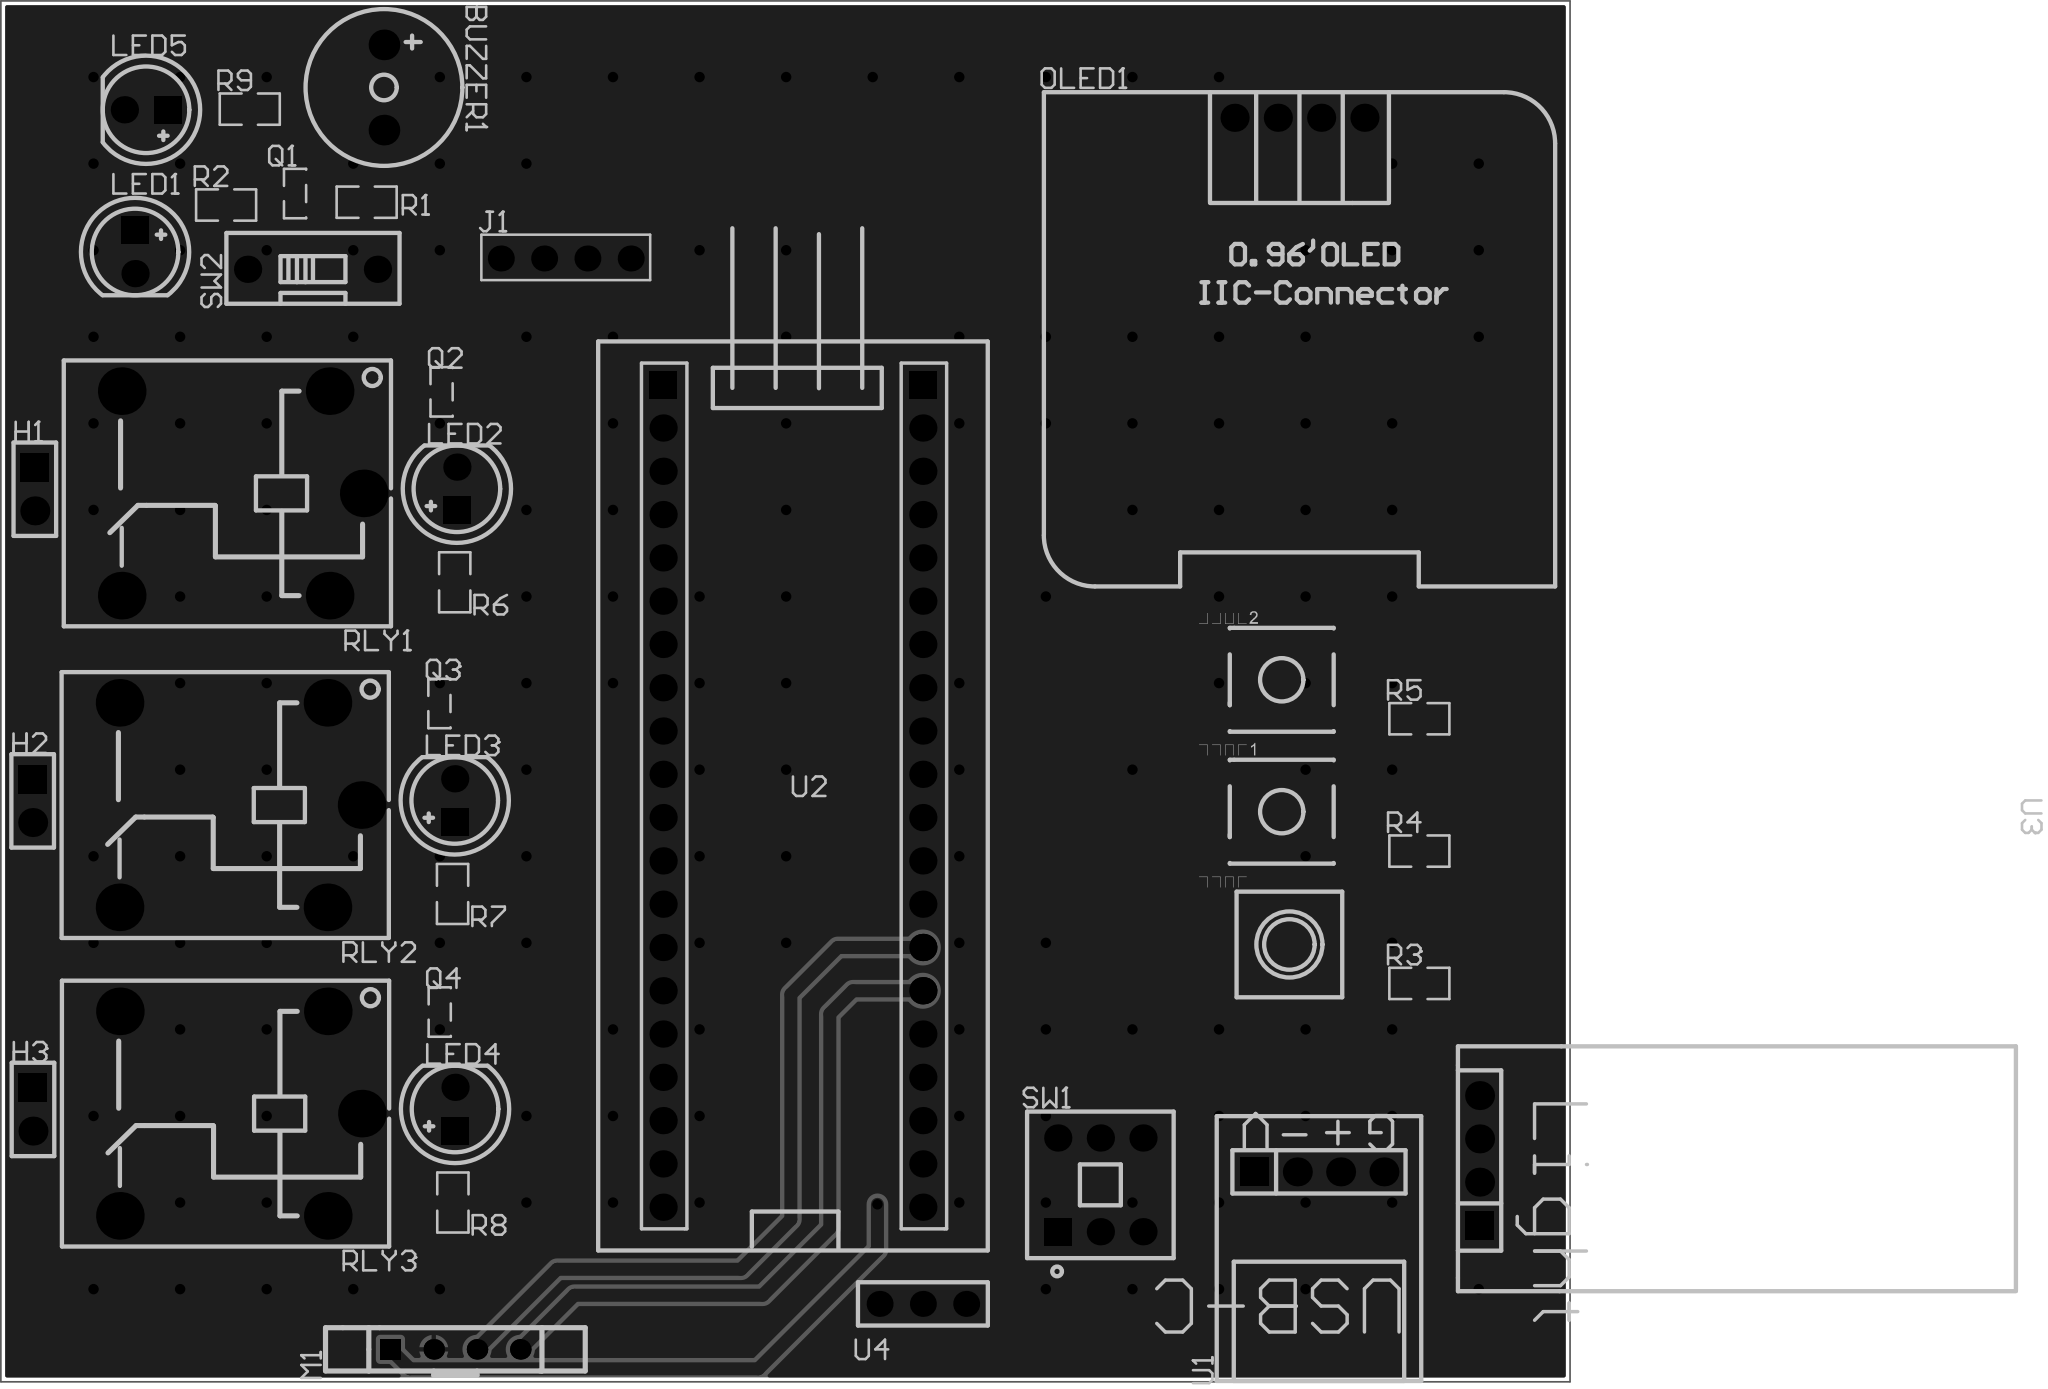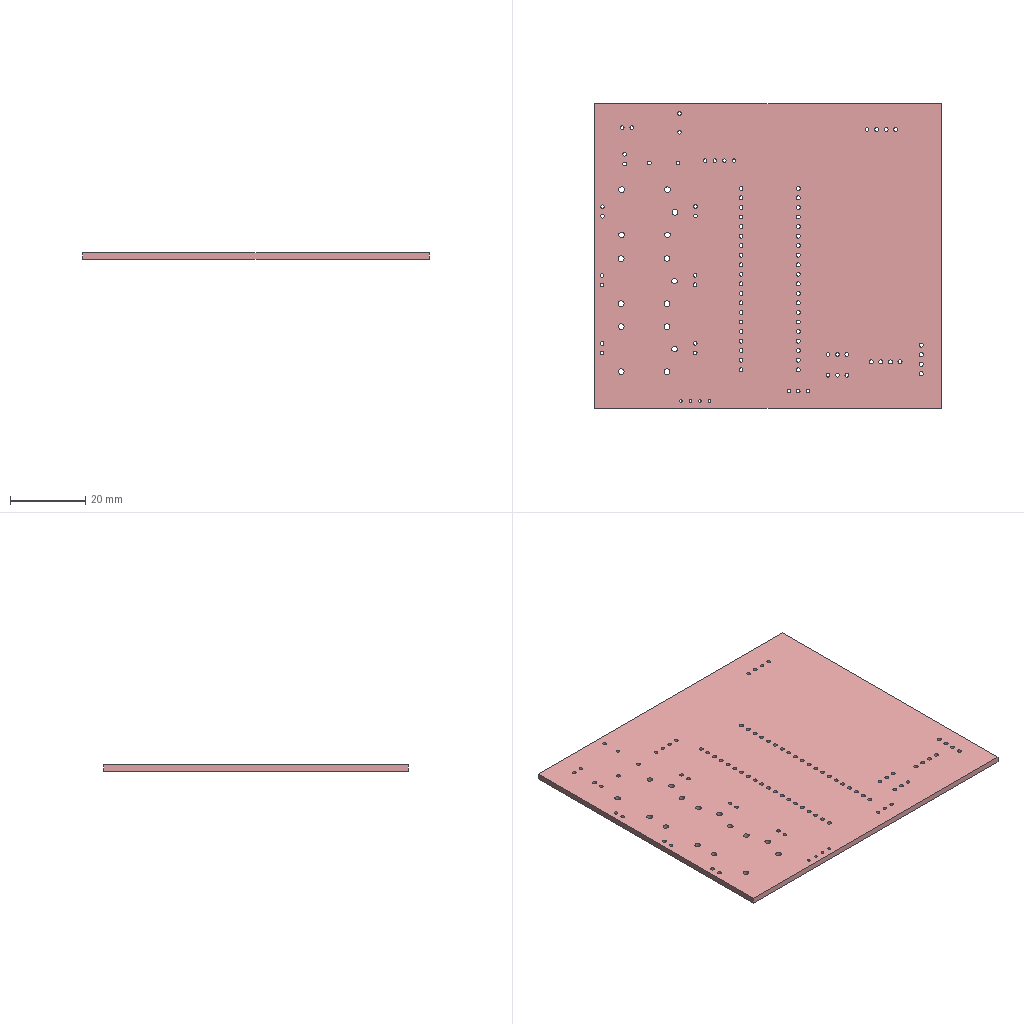Circuit board layout | Altium Designer | box 92.1 x 81 x 1.6 mm
Layer stack:
# Altium Designer layer stack of  (unit mm; dielectric type: 0 none, 1 core, 2 prepreg, 3 surface material)
index,name,kind,layer,copper_thickness_mm,dielectric_type,dielectric_thickness_mm,dielectric_material,dielectric_constant
0,Top Paste Mask Layer,other,,,,,,
1,Top Silkscreen Layer,other,,,,,,
2,Top Solder Mask Layer,dielectric,,,3,0.01,,3.3
3,Top Layer,copper,Top Layer,0.035,,,,
4,Dielectric1,dielectric,,,3,1.51,FR4,4.5
5,Bottom Layer,copper,Bottom Layer,0.035,,,,
6,Bottom Solder Mask Layer,dielectric,,,3,0.01,,3.3
7,Bottom Silkscreen Layer,other,,,,,,
8,Bottom Paste Mask Layer,other,,,,,,
# drill layer pairs: low layer,high layer
drill_pair,Top Layer,Bottom Layer
Part placement:
Designator,Comment,Layer,Footprint,Center-X(mm),Center-Y(mm),Rotation
BUZZER1,3kHz,TopLayer,BUZ-TH_BD9.0-P5.00-D0.6-FD,102.997,157.988,270
H1,,TopLayer,HDR-TH_2P-P2.54-V-F,82.511,134.416,270
H2,,TopLayer,HDR-TH_2P-P2.54-V-F,82.385,116.128,270
H3,,TopLayer,HDR-TH_2P-P2.54-V-F,82.403,98.024,270
J1,土壤湿度传感器模块,TopLayer,Hearder-4,113.665,147.955,0
LED1,,TopLayer,LED-TH_5mm,88.392,148.336,270
LED2,,TopLayer,LED-TH_5mm,107.276,134.443,90
LED3,,TopLayer,LED-TH_5mm,107.15,116.155,90
LED4,,TopLayer,LED-TH_5mm,107.168,98.051,90
LED5,,TopLayer,LED-TH_5mm,89.036,156.68,180
M1,BT06,TopLayer,BT06,107.188,83.947,90
OLED1,,TopLayer,0.96OLED_4P,156.718,156.21,0
Q1,S8050,TopLayer,SOT-23-3_L2.9-W1.3-P1.90-LS2.3-BR,97.79,151.765,0
Q2,S8050,TopLayer,SOT-23-3_L2.9-W1.3-P1.90-LS2.3-BR,106.388,140.131,0
Q3,S8050,TopLayer,SOT-23-3_L2.9-W1.3-P1.90-LS2.3-BR,106.26,121.843,0
Q4,S8050,TopLayer,SOT-23-3_L2.9-W1.3-P1.90-LS2.3-BR,106.279,103.739,0
R1,1K,TopLayer,R0805,101.981,151.257,180
R2,1K,TopLayer,R0805,93.735,151.092,0
R3,10K,TopLayer,R0805,163.752,105.418,0
R4,10K,TopLayer,R0805,163.752,113.183,0
R5,10K,TopLayer,R0805,163.752,120.948,0
R6,1K,TopLayer,R0805,107.15,128.955,90
R7,1K,TopLayer,R0805,107.022,110.667,90
R8,1K,TopLayer,R0805,107.041,92.563,90
R9,1K,TopLayer,R0805,95.123,156.718,0
RLY1,SRD-05VDC-SL-C,TopLayer,RELAY-TH_SRD-XXVDC-XL-C,94.71,134.172,180
RLY2,SRD-05VDC-SL-C,TopLayer,RELAY-TH_SRD-XXVDC-XL-C,94.583,115.884,180
RLY3,SRD-05VDC-SL-C,TopLayer,RELAY-TH_SRD-XXVDC-XL-C,94.602,97.78,180
SW1,自锁开关,TopLayer,SW-TH_6P-L8.5-W8.5-P2.50-LS5.5-BL-2,145.034,93.599,0
SW2,拨码,TopLayer,SW-TH_DSWB01LHGET,98.806,147.32,90
U1,,TopLayer,USB-type-C模块,157.861,94.361,90
U2,CW32F030C8最小系统板,TopLayer,STM32F103C8T6核心板,126.996,116.418,0
U3,,TopLayer,光敏传感器模块,167.285,95.027,270
U4,DS18B20,TopLayer,3p_2.54,134.62,86.614,0
轻触按键,SH-6X6X6.5H-TP,TopLayer,SW-SMD_4P-L6.2-W6.2-P4.50-LS9.5-TL,156.126,107.704,0
轻触按键1,SH-6X6X6.5H-TP,TopLayer,SW-SMD_4P-L6.0-W6.0-P4.50-LS8.8,155.676,115.495,0
轻触按键2,SH-6X6X6.5H-TP,TopLayer,SW-SMD_4P-L6.0-W6.0-P4.50-LS8.8,155.676,123.234,0
Pad and via stacks:
# Altium Designer via and pad stacks of  (unit mm). Each distinct definition once, with the count of objects using it.
# via: kind,start_layer,end_layer,hole_mm,diameter_mm,mode(0 simple;1 top-mid-bottom;2 full stack),diameter_per_layer,count,example_net
# pad: kind,layer,hole_mm,hole_type(0 round;1 square;2 slot),plating,top_size,top_shape(1 round;2 rect;3 octagon;9 rounded rect),mid_size,bottom_size,mode,footprint,size_per_layer,count,example
pad,Multi-Layer,1,0,plated,1.8x1.8,1,1.8x1.8,1.8x1.8,0,BUZ-TH_BD9.0-P5.00-D0.6-FD,,2,BUZZER1.1
pad,Multi-Layer,1,0,plated,1.7x1.7,2,1.7x1.7,1.7x1.7,0,HDR-TH_2P-P2.54-V-F,,3,H1.1
pad,Multi-Layer,1,0,plated,1.7x1.7,1,1.7x1.7,1.7x1.7,0,HDR-TH_2P-P2.54-V-F,,3,H1.2
pad,Multi-Layer,0.9144,0,plated,1.524x1.524,1,1.524x1.524,1.524x1.524,0,Hearder-4,,4,J1.1
pad,Multi-Layer,1,0,plated,1.6x1.6,2,1.6x1.6,1.6x1.6,0,LED-TH_5mm,,5,LED1.1
pad,Multi-Layer,1,0,plated,1.6x1.6,1,1.6x1.6,1.6x1.6,0,LED-TH_5mm,,5,LED1.2
pad,Multi-Layer,0.7,0,plated,1.2x1.2,2,1.2x1.2,1.2x1.2,0,BT06,,1,M1.1
pad,Multi-Layer,0.7,0,plated,1.2x1.2,1,1.2x1.2,1.2x1.2,0,BT06,,3,M1.2
pad,Multi-Layer,1,0,plated,1.65x1.65,1,1.65x1.65,1.65x1.65,0,0.96OLED_4P,,4,OLED1.4
pad,Multi-Layer,1.524,0,plated,2.794x2.794,1,2.794x2.794,2.794x2.794,0,RELAY-TH_SRD-XXVDC-XL-C,,15,RLY1.2
pad,Multi-Layer,1,0,plated,1.6x1.6,2,1.6x1.6,1.6x1.6,0,SW-TH_6P-L8.5-W8.5-P2.50-LS5.5-BL-2,,1,SW1.1
pad,Multi-Layer,1,0,plated,1.6x1.6,1,1.6x1.6,1.6x1.6,0,SW-TH_6P-L8.5-W8.5-P2.50-LS5.5-BL-2,,5,SW1.2
pad,Multi-Layer,1,0,plated,1.6x1.6,1,1.6x1.6,1.6x1.6,0,SW-TH_DSWB01LHGET,,2,SW2.2
pad,Multi-Layer,1.1,0,plated,1.7x1.7,2,1.7x1.7,1.7x1.7,0,USB-type-C\u00C4\u00A3\u00BF\u00E9,,1,U1.1
pad,Multi-Layer,1.1,0,plated,1.7x1.7,1,1.7x1.7,1.7x1.7,0,USB-type-C\u00C4\u00A3\u00BF\u00E9,,3,U1.2
pad,Multi-Layer,1.049,0,plated,1.6x1.6,2,1.6x1.6,1.6x1.6,0,STM32F103C8T6\u00BA\u00CB\u00D0\u00C4\u00B0\u00E5,,2,U2.1
pad,Multi-Layer,1.049,0,plated,1.6x1.6,1,1.6x1.6,1.6x1.6,0,STM32F103C8T6\u00BA\u00CB\u00D0\u00C4\u00B0\u00E5,,38,U2.2
pad,Multi-Layer,1.1,0,plated,1.7x1.7,2,1.7x1.7,1.7x1.7,0,\u00B9\u00E2\u00C3\u00F4\u00B4\u00AB\u00B8\u00D0\u00C6\u00F7\u00C4\u00A3\u00BF\u00E9,,1,U3.1
pad,Multi-Layer,1.1,0,plated,1.7x1.7,1,1.7x1.7,1.7x1.7,0,\u00B9\u00E2\u00C3\u00F4\u00B4\u00AB\u00B8\u00D0\u00C6\u00F7\u00C4\u00A3\u00BF\u00E9,,3,U3.2
pad,Multi-Layer,0.9144,0,plated,1.524x1.524,1,1.524x1.524,1.524x1.524,0,3p_2.54,,3,U4.1
pad,Top Layer,0,0,plated,1.07x0.532,2,1.07x0.532,1.07x0.532,0,SOT-23-3_L2.9-W1.3-P1.90-LS2.3-BR,,12,Q1.3
pad,Top Layer,0,0,plated,1.133x1.377,2,1.133x1.377,1.133x1.377,0,R0805,,18,R1.2
pad,Top Layer,0,0,plated,1.8x1.3,2,1.8x1.3,1.8x1.3,0,SW-SMD_4P-L6.2-W6.2-P4.50-LS9.5-TL,,4,\u8F7B\u89E6\u6309\u952E.1
pad,Top Layer,0,0,plated,1.7x1.1,2,1.7x1.1,1.7x1.1,0,SW-SMD_4P-L6.0-W6.0-P4.50-LS8.8,,8,\u8F7B\u89E6\u6309\u952E1.4
via,Top Layer,Bottom Layer,0.3048,0.61,0,,159,+5V
Copper pours:
name,layer,net,type(0 solid;1 hatched;2 none)
Top Layer-GND,Top Layer,GND,0
Bottom Layer-GND,Bottom Layer,GND,0